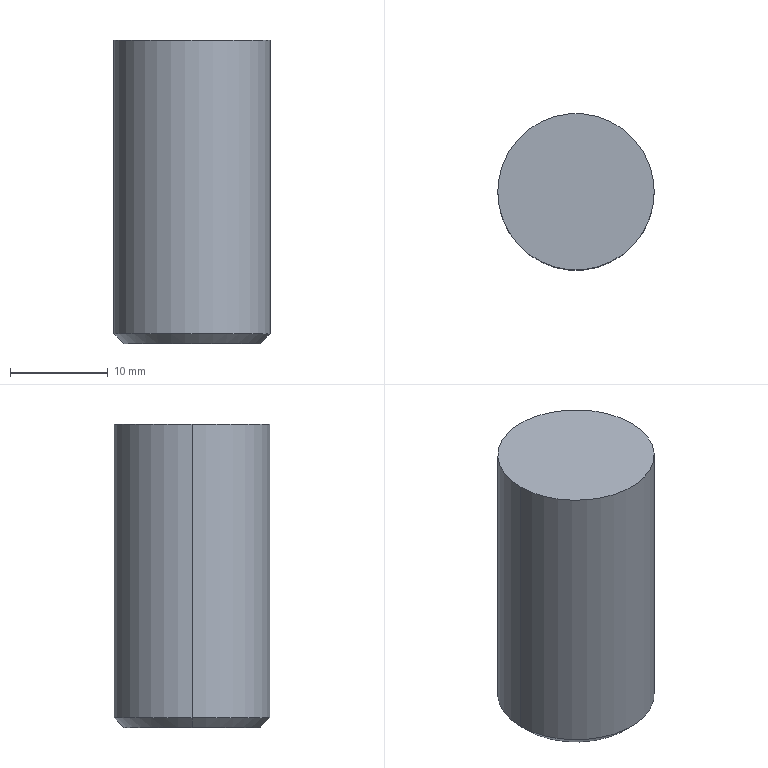Part | SolidWorks | features Chamfer 1, Extrusion 1 | 1 solid | 6 faces | box 16 x 16 x 31 mm | volume 6209 mm3 | cone 2 | cylinder 2 | plane 2 | commonest cylinder face diameters 16 x2
STEP:
#1=CARTESIAN_POINT('',(-7.,0.,0.));
#2=VERTEX_POINT('',#1);
#3=CARTESIAN_POINT('',(7.,0.,0.));
#4=VERTEX_POINT('',#3);
#5=CARTESIAN_POINT('',(0.,0.,0.));
#6=DIRECTION('',(0.,0.,-1.));
#7=DIRECTION('',(1.,0.,0.));
#8=AXIS2_PLACEMENT_3D('',#5,#6,#7);
#9=CIRCLE('',#8,7.);
#10=EDGE_CURVE('',#2,#4,#9,.T.);
#11=ORIENTED_EDGE('',*,*,#10,.F.);
#12=CARTESIAN_POINT('',(-8.,0.,1.));
#13=VERTEX_POINT('',#12);
#14=CARTESIAN_POINT('',(-8.,0.,1.));
#15=DIRECTION('',(-0.7071,0.,0.7071));
#16=VECTOR('',#15,1000.);
#17=LINE('',#14,#16);
#18=EDGE_CURVE('',#2,#13,#17,.T.);
#19=ORIENTED_EDGE('',*,*,#18,.T.);
#20=CARTESIAN_POINT('',(8.,0.,1.));
#21=VERTEX_POINT('',#20);
#22=CARTESIAN_POINT('',(0.,0.,1.));
#23=DIRECTION('',(0.,0.,1.));
#24=DIRECTION('',(1.,0.,0.));
#25=AXIS2_PLACEMENT_3D('',#22,#23,#24);
#26=CIRCLE('',#25,8.);
#27=EDGE_CURVE('',#21,#13,#26,.T.);
#28=ORIENTED_EDGE('',*,*,#27,.F.);
#29=CARTESIAN_POINT('',(8.,0.,1.));
#30=DIRECTION('',(0.7071,0.,0.7071));
#31=VECTOR('',#30,1000.);
#32=LINE('',#29,#31);
#33=EDGE_CURVE('',#4,#21,#32,.T.);
#34=ORIENTED_EDGE('',*,*,#33,.F.);
#35=EDGE_LOOP('',(#11,#19,#28,#34));
#36=FACE_OUTER_BOUND('',#35,.T.);
#37=CARTESIAN_POINT('',(0.,0.,1.));
#38=DIRECTION('',(0.,0.,1.));
#39=DIRECTION('',(1.,0.,0.));
#40=AXIS2_PLACEMENT_3D('',#37,#38,#39);
#41=CONICAL_SURFACE('',#40,8.,0.7854);
#42=ADVANCED_FACE('',(#36),#41,.T.);
#43=CARTESIAN_POINT('',(8.,0.,31.));
#44=VERTEX_POINT('',#43);
#45=CARTESIAN_POINT('',(-8.,0.,31.));
#46=VERTEX_POINT('',#45);
#47=CARTESIAN_POINT('',(0.,0.,31.));
#48=DIRECTION('',(0.,0.,1.));
#49=DIRECTION('',(1.,0.,0.));
#50=AXIS2_PLACEMENT_3D('',#47,#48,#49);
#51=CIRCLE('',#50,8.);
#52=EDGE_CURVE('',#44,#46,#51,.T.);
#53=ORIENTED_EDGE('',*,*,#52,.F.);
#54=CARTESIAN_POINT('',(8.,0.,31.));
#55=DIRECTION('',(0.,0.,-1.));
#56=VECTOR('',#55,1000.);
#57=LINE('',#54,#56);
#58=EDGE_CURVE('',#44,#21,#57,.T.);
#59=ORIENTED_EDGE('',*,*,#58,.T.);
#60=ORIENTED_EDGE('',*,*,#27,.T.);
#61=CARTESIAN_POINT('',(-8.,0.,31.));
#62=DIRECTION('',(0.,0.,-1.));
#63=VECTOR('',#62,1000.);
#64=LINE('',#61,#63);
#65=EDGE_CURVE('',#46,#13,#64,.T.);
#66=ORIENTED_EDGE('',*,*,#65,.F.);
#67=EDGE_LOOP('',(#53,#59,#60,#66));
#68=FACE_OUTER_BOUND('',#67,.T.);
#69=CARTESIAN_POINT('',(0.,0.,31.));
#70=DIRECTION('',(0.,0.,-1.));
#71=DIRECTION('',(-1.,0.,0.));
#72=AXIS2_PLACEMENT_3D('',#69,#70,#71);
#73=CYLINDRICAL_SURFACE('',#72,8.);
#74=ADVANCED_FACE('',(#68),#73,.T.);
#75=ORIENTED_EDGE('',*,*,#58,.F.);
#76=CARTESIAN_POINT('',(0.,0.,31.));
#77=DIRECTION('',(0.,0.,1.));
#78=DIRECTION('',(1.,0.,0.));
#79=AXIS2_PLACEMENT_3D('',#76,#77,#78);
#80=CIRCLE('',#79,8.);
#81=EDGE_CURVE('',#46,#44,#80,.T.);
#82=ORIENTED_EDGE('',*,*,#81,.F.);
#83=ORIENTED_EDGE('',*,*,#65,.T.);
#84=CARTESIAN_POINT('',(0.,0.,1.));
#85=DIRECTION('',(0.,0.,1.));
#86=DIRECTION('',(1.,0.,0.));
#87=AXIS2_PLACEMENT_3D('',#84,#85,#86);
#88=CIRCLE('',#87,8.);
#89=EDGE_CURVE('',#13,#21,#88,.T.);
#90=ORIENTED_EDGE('',*,*,#89,.T.);
#91=EDGE_LOOP('',(#75,#82,#83,#90));
#92=FACE_OUTER_BOUND('',#91,.T.);
#93=CARTESIAN_POINT('',(0.,0.,31.));
#94=DIRECTION('',(0.,0.,-1.));
#95=DIRECTION('',(-1.,0.,0.));
#96=AXIS2_PLACEMENT_3D('',#93,#94,#95);
#97=CYLINDRICAL_SURFACE('',#96,8.);
#98=ADVANCED_FACE('',(#92),#97,.T.);
#99=ORIENTED_EDGE('',*,*,#81,.T.);
#100=ORIENTED_EDGE('',*,*,#52,.T.);
#101=EDGE_LOOP('',(#99,#100));
#102=FACE_OUTER_BOUND('',#101,.T.);
#103=CARTESIAN_POINT('',(0.,0.,31.));
#104=DIRECTION('',(0.,0.,1.));
#105=DIRECTION('',(1.,0.,0.));
#106=AXIS2_PLACEMENT_3D('',#103,#104,#105);
#107=PLANE('',#106);
#108=ADVANCED_FACE('',(#102),#107,.T.);
#109=CARTESIAN_POINT('',(0.,0.,0.));
#110=DIRECTION('',(0.,0.,-1.));
#111=DIRECTION('',(1.,0.,0.));
#112=AXIS2_PLACEMENT_3D('',#109,#110,#111);
#113=CIRCLE('',#112,7.);
#114=EDGE_CURVE('',#4,#2,#113,.T.);
#115=ORIENTED_EDGE('',*,*,#114,.T.);
#116=ORIENTED_EDGE('',*,*,#10,.T.);
#117=EDGE_LOOP('',(#115,#116));
#118=FACE_OUTER_BOUND('',#117,.T.);
#119=CARTESIAN_POINT('',(0.,0.,0.));
#120=DIRECTION('',(0.,0.,1.));
#121=DIRECTION('',(1.,0.,0.));
#122=AXIS2_PLACEMENT_3D('',#119,#120,#121);
#123=PLANE('',#122);
#124=ADVANCED_FACE('',(#118),#123,.F.);
#125=ORIENTED_EDGE('',*,*,#18,.F.);
#126=ORIENTED_EDGE('',*,*,#114,.F.);
#127=ORIENTED_EDGE('',*,*,#33,.T.);
#128=ORIENTED_EDGE('',*,*,#89,.F.);
#129=EDGE_LOOP('',(#125,#126,#127,#128));
#130=FACE_OUTER_BOUND('',#129,.T.);
#131=CARTESIAN_POINT('',(0.,0.,1.));
#132=DIRECTION('',(0.,0.,1.));
#133=DIRECTION('',(1.,0.,0.));
#134=AXIS2_PLACEMENT_3D('',#131,#132,#133);
#135=CONICAL_SURFACE('',#134,8.,0.7854);
#136=ADVANCED_FACE('',(#130),#135,.T.);
#137=CLOSED_SHELL('',(#42,#74,#98,#108,#124,#136));
#138=MANIFOLD_SOLID_BREP('',#137);
#139=CARTESIAN_POINT('',(0.,0.,0.));
#140=DIRECTION('',(0.,0.,1.));
#141=DIRECTION('',(1.,0.,0.));
#142=AXIS2_PLACEMENT_3D('',#139,#140,#141);
#143=(LENGTH_UNIT()NAMED_UNIT(*)SI_UNIT(.MILLI.,.METRE.));
#144=UNCERTAINTY_MEASURE_WITH_UNIT(LENGTH_MEASURE(0.00001),#143,'','');
#145=(NAMED_UNIT(*)PLANE_ANGLE_UNIT()SI_UNIT($,.RADIAN.));
#146=(NAMED_UNIT(*)SI_UNIT($,.STERADIAN.)SOLID_ANGLE_UNIT());
#147=(GEOMETRIC_REPRESENTATION_CONTEXT(3)GLOBAL_UNCERTAINTY_ASSIGNED_CONTEXT((#144))GLOBAL_UNIT_ASSIGNED_CONTEXT((#143,#145,#146))REPRESENTATION_CONTEXT('',''));
#148=ADVANCED_BREP_SHAPE_REPRESENTATION('',(#138,#142),#147);